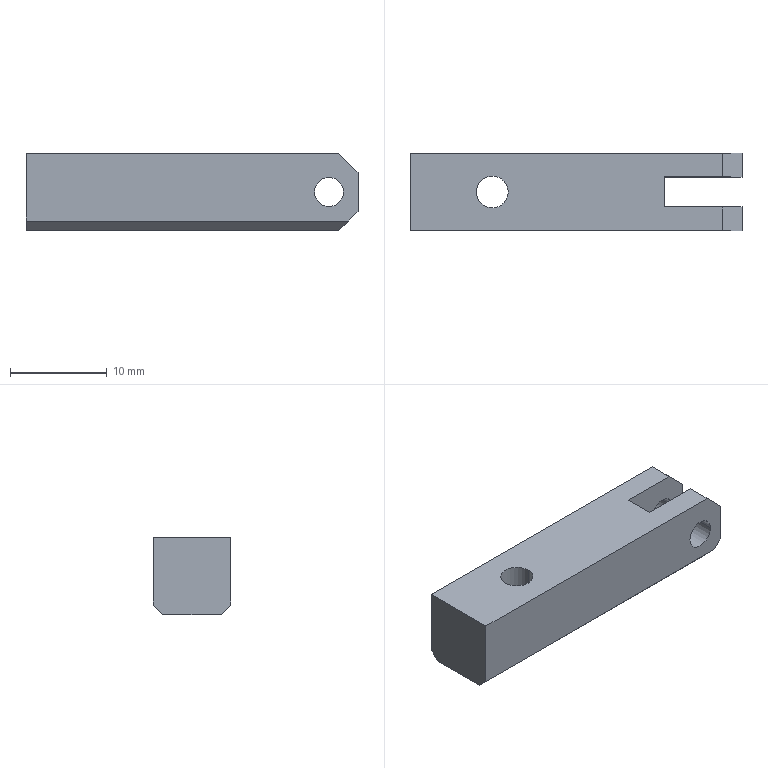Part | NX | features BREP 1 | 1 solid | 22 faces | box 34.3 x 8 x 8 mm | volume 1842 mm3 | plane 16 | cylinder 6 | commonest cylinder face diameters 3 x4 3.3 x2
STEP:
#1=CARTESIAN_POINT('',(-742.945,57.566,0.));
#2=VERTEX_POINT('',#1);
#3=CARTESIAN_POINT('',(-739.645,57.566,0.));
#4=VERTEX_POINT('',#3);
#5=CARTESIAN_POINT('',(-741.295,57.566,0.));
#6=DIRECTION('',(0.,0.,1.));
#7=DIRECTION('',(1.,0.,0.));
#8=AXIS2_PLACEMENT_3D('',#5,#6,#7);
#9=CIRCLE('',#8,1.65);
#10=EDGE_CURVE('',#2,#4,#9,.T.);
#11=ORIENTED_EDGE('',*,*,#10,.F.);
#12=CARTESIAN_POINT('',(-742.945,57.566,8.));
#13=VERTEX_POINT('',#12);
#14=CARTESIAN_POINT('',(-742.945,57.566,8.));
#15=DIRECTION('',(0.,0.,1.));
#16=VECTOR('',#15,1000.);
#17=LINE('',#14,#16);
#18=EDGE_CURVE('',#13,#2,#17,.F.);
#19=ORIENTED_EDGE('',*,*,#18,.F.);
#20=CARTESIAN_POINT('',(-739.645,57.566,8.));
#21=VERTEX_POINT('',#20);
#22=CARTESIAN_POINT('',(-741.295,57.566,8.));
#23=DIRECTION('',(0.,0.,1.));
#24=DIRECTION('',(1.,0.,0.));
#25=AXIS2_PLACEMENT_3D('',#22,#23,#24);
#26=CIRCLE('',#25,1.65);
#27=EDGE_CURVE('',#13,#21,#26,.T.);
#28=ORIENTED_EDGE('',*,*,#27,.T.);
#29=CARTESIAN_POINT('',(-739.645,57.566,8.));
#30=DIRECTION('',(0.,0.,1.));
#31=VECTOR('',#30,1000.);
#32=LINE('',#29,#31);
#33=EDGE_CURVE('',#21,#4,#32,.F.);
#34=ORIENTED_EDGE('',*,*,#33,.T.);
#35=EDGE_LOOP('',(#11,#19,#28,#34));
#36=FACE_BOUND('',#35,.T.);
#37=CARTESIAN_POINT('',(-741.295,57.566,8.));
#38=DIRECTION('',(0.,0.,1.));
#39=DIRECTION('',(1.,0.,0.));
#40=AXIS2_PLACEMENT_3D('',#37,#38,#39);
#41=CYLINDRICAL_SURFACE('',#40,1.65);
#42=ADVANCED_FACE('',(#36),#41,.F.);
#43=CARTESIAN_POINT('',(-719.995,56.016,4.));
#44=VERTEX_POINT('',#43);
#45=CARTESIAN_POINT('',(-716.995,56.016,4.));
#46=VERTEX_POINT('',#45);
#47=CARTESIAN_POINT('',(-718.495,56.016,4.));
#48=DIRECTION('',(0.,-1.,0.));
#49=DIRECTION('',(1.,0.,0.));
#50=AXIS2_PLACEMENT_3D('',#47,#48,#49);
#51=CIRCLE('',#50,1.5);
#52=EDGE_CURVE('',#44,#46,#51,.T.);
#53=ORIENTED_EDGE('',*,*,#52,.F.);
#54=CARTESIAN_POINT('',(-719.995,53.566,4.));
#55=VERTEX_POINT('',#54);
#56=CARTESIAN_POINT('',(-719.995,61.566,4.));
#57=DIRECTION('',(0.,-1.,0.));
#58=VECTOR('',#57,1000.);
#59=LINE('',#56,#58);
#60=EDGE_CURVE('',#55,#44,#59,.F.);
#61=ORIENTED_EDGE('',*,*,#60,.F.);
#62=CARTESIAN_POINT('',(-716.995,53.566,4.));
#63=VERTEX_POINT('',#62);
#64=CARTESIAN_POINT('',(-718.495,53.566,4.));
#65=DIRECTION('',(0.,-1.,0.));
#66=DIRECTION('',(1.,0.,0.));
#67=AXIS2_PLACEMENT_3D('',#64,#65,#66);
#68=CIRCLE('',#67,1.5);
#69=EDGE_CURVE('',#55,#63,#68,.T.);
#70=ORIENTED_EDGE('',*,*,#69,.T.);
#71=CARTESIAN_POINT('',(-716.995,61.566,4.));
#72=DIRECTION('',(0.,-1.,0.));
#73=VECTOR('',#72,1000.);
#74=LINE('',#71,#73);
#75=EDGE_CURVE('',#63,#46,#74,.F.);
#76=ORIENTED_EDGE('',*,*,#75,.T.);
#77=EDGE_LOOP('',(#53,#61,#70,#76));
#78=FACE_BOUND('',#77,.T.);
#79=CARTESIAN_POINT('',(-718.495,61.566,4.));
#80=DIRECTION('',(0.,-1.,0.));
#81=DIRECTION('',(1.,0.,0.));
#82=AXIS2_PLACEMENT_3D('',#79,#80,#81);
#83=CYLINDRICAL_SURFACE('',#82,1.5);
#84=ADVANCED_FACE('',(#78),#83,.F.);
#85=CARTESIAN_POINT('',(-719.995,61.566,4.));
#86=VERTEX_POINT('',#85);
#87=CARTESIAN_POINT('',(-716.995,61.566,4.));
#88=VERTEX_POINT('',#87);
#89=CARTESIAN_POINT('',(-718.495,61.566,4.));
#90=DIRECTION('',(0.,-1.,0.));
#91=DIRECTION('',(1.,0.,0.));
#92=AXIS2_PLACEMENT_3D('',#89,#90,#91);
#93=CIRCLE('',#92,1.5);
#94=EDGE_CURVE('',#86,#88,#93,.T.);
#95=ORIENTED_EDGE('',*,*,#94,.F.);
#96=CARTESIAN_POINT('',(-719.995,59.116,4.));
#97=VERTEX_POINT('',#96);
#98=CARTESIAN_POINT('',(-719.995,61.566,4.));
#99=DIRECTION('',(0.,-1.,0.));
#100=VECTOR('',#99,1000.);
#101=LINE('',#98,#100);
#102=EDGE_CURVE('',#97,#86,#101,.F.);
#103=ORIENTED_EDGE('',*,*,#102,.F.);
#104=CARTESIAN_POINT('',(-716.995,59.116,4.));
#105=VERTEX_POINT('',#104);
#106=CARTESIAN_POINT('',(-718.495,59.116,4.));
#107=DIRECTION('',(0.,1.,0.));
#108=DIRECTION('',(-1.,0.,0.));
#109=AXIS2_PLACEMENT_3D('',#106,#107,#108);
#110=CIRCLE('',#109,1.5);
#111=EDGE_CURVE('',#105,#97,#110,.T.);
#112=ORIENTED_EDGE('',*,*,#111,.F.);
#113=CARTESIAN_POINT('',(-716.995,61.566,4.));
#114=DIRECTION('',(0.,-1.,0.));
#115=VECTOR('',#114,1000.);
#116=LINE('',#113,#115);
#117=EDGE_CURVE('',#105,#88,#116,.F.);
#118=ORIENTED_EDGE('',*,*,#117,.T.);
#119=EDGE_LOOP('',(#95,#103,#112,#118));
#120=FACE_BOUND('',#119,.T.);
#121=CARTESIAN_POINT('',(-718.495,61.566,4.));
#122=DIRECTION('',(0.,-1.,0.));
#123=DIRECTION('',(1.,0.,0.));
#124=AXIS2_PLACEMENT_3D('',#121,#122,#123);
#125=CYLINDRICAL_SURFACE('',#124,1.5);
#126=ADVANCED_FACE('',(#120),#125,.F.);
#127=CARTESIAN_POINT('',(-715.495,53.566,6.));
#128=VERTEX_POINT('',#127);
#129=CARTESIAN_POINT('',(-715.495,53.566,2.));
#130=VERTEX_POINT('',#129);
#131=CARTESIAN_POINT('',(-715.495,53.566,8.));
#132=DIRECTION('',(0.,0.,-1.));
#133=VECTOR('',#132,1000.);
#134=LINE('',#131,#133);
#135=EDGE_CURVE('',#128,#130,#134,.T.);
#136=ORIENTED_EDGE('',*,*,#135,.T.);
#137=CARTESIAN_POINT('',(-715.495,56.016,2.));
#138=VERTEX_POINT('',#137);
#139=CARTESIAN_POINT('',(-715.495,53.566,2.));
#140=DIRECTION('',(0.,1.,0.));
#141=VECTOR('',#140,1000.);
#142=LINE('',#139,#141);
#143=EDGE_CURVE('',#130,#138,#142,.T.);
#144=ORIENTED_EDGE('',*,*,#143,.T.);
#145=CARTESIAN_POINT('',(-715.495,56.016,6.));
#146=VERTEX_POINT('',#145);
#147=CARTESIAN_POINT('',(-715.495,56.016,0.));
#148=DIRECTION('',(0.,0.,1.));
#149=VECTOR('',#148,1000.);
#150=LINE('',#147,#149);
#151=EDGE_CURVE('',#138,#146,#150,.T.);
#152=ORIENTED_EDGE('',*,*,#151,.T.);
#153=CARTESIAN_POINT('',(-715.495,53.566,6.));
#154=DIRECTION('',(0.,-1.,0.));
#155=VECTOR('',#154,1000.);
#156=LINE('',#153,#155);
#157=EDGE_CURVE('',#146,#128,#156,.T.);
#158=ORIENTED_EDGE('',*,*,#157,.T.);
#159=EDGE_LOOP('',(#136,#144,#152,#158));
#160=FACE_BOUND('',#159,.T.);
#161=CARTESIAN_POINT('',(-715.495,53.566,8.));
#162=DIRECTION('',(-1.,0.,0.));
#163=DIRECTION('',(0.,0.,1.));
#164=AXIS2_PLACEMENT_3D('',#161,#162,#163);
#165=PLANE('',#164);
#166=ADVANCED_FACE('',(#160),#165,.F.);
#167=CARTESIAN_POINT('',(-715.495,59.116,2.));
#168=VERTEX_POINT('',#167);
#169=CARTESIAN_POINT('',(-715.495,59.116,6.));
#170=VERTEX_POINT('',#169);
#171=CARTESIAN_POINT('',(-715.495,59.116,0.));
#172=DIRECTION('',(0.,0.,1.));
#173=VECTOR('',#172,1000.);
#174=LINE('',#171,#173);
#175=EDGE_CURVE('',#168,#170,#174,.T.);
#176=ORIENTED_EDGE('',*,*,#175,.F.);
#177=CARTESIAN_POINT('',(-715.495,61.566,2.));
#178=VERTEX_POINT('',#177);
#179=CARTESIAN_POINT('',(-715.495,53.566,2.));
#180=DIRECTION('',(0.,1.,0.));
#181=VECTOR('',#180,1000.);
#182=LINE('',#179,#181);
#183=EDGE_CURVE('',#168,#178,#182,.T.);
#184=ORIENTED_EDGE('',*,*,#183,.T.);
#185=CARTESIAN_POINT('',(-715.495,61.566,6.));
#186=VERTEX_POINT('',#185);
#187=CARTESIAN_POINT('',(-715.495,61.566,8.));
#188=DIRECTION('',(0.,0.,-1.));
#189=VECTOR('',#188,1000.);
#190=LINE('',#187,#189);
#191=EDGE_CURVE('',#186,#178,#190,.T.);
#192=ORIENTED_EDGE('',*,*,#191,.F.);
#193=CARTESIAN_POINT('',(-715.495,59.116,6.));
#194=DIRECTION('',(0.,-1.,0.));
#195=VECTOR('',#194,1000.);
#196=LINE('',#193,#195);
#197=EDGE_CURVE('',#186,#170,#196,.T.);
#198=ORIENTED_EDGE('',*,*,#197,.T.);
#199=EDGE_LOOP('',(#176,#184,#192,#198));
#200=FACE_BOUND('',#199,.T.);
#201=CARTESIAN_POINT('',(-715.495,53.566,8.));
#202=DIRECTION('',(-1.,0.,0.));
#203=DIRECTION('',(0.,0.,1.));
#204=AXIS2_PLACEMENT_3D('',#201,#202,#203);
#205=PLANE('',#204);
#206=ADVANCED_FACE('',(#200),#205,.F.);
#207=CARTESIAN_POINT('',(-716.495,61.566,1.));
#208=VERTEX_POINT('',#207);
#209=CARTESIAN_POINT('',(-715.495,61.566,2.));
#210=DIRECTION('',(-0.7071,0.,-0.7071));
#211=VECTOR('',#210,1000.);
#212=LINE('',#209,#211);
#213=EDGE_CURVE('',#178,#208,#212,.T.);
#214=ORIENTED_EDGE('',*,*,#213,.T.);
#215=CARTESIAN_POINT('',(-749.795,61.566,1.));
#216=VERTEX_POINT('',#215);
#217=CARTESIAN_POINT('',(-715.495,61.566,1.));
#218=DIRECTION('',(-1.,0.,0.));
#219=VECTOR('',#218,1000.);
#220=LINE('',#217,#219);
#221=EDGE_CURVE('',#208,#216,#220,.T.);
#222=ORIENTED_EDGE('',*,*,#221,.T.);
#223=CARTESIAN_POINT('',(-749.795,61.566,8.));
#224=VERTEX_POINT('',#223);
#225=CARTESIAN_POINT('',(-749.795,61.566,8.));
#226=DIRECTION('',(0.,0.,-1.));
#227=VECTOR('',#226,1000.);
#228=LINE('',#225,#227);
#229=EDGE_CURVE('',#224,#216,#228,.T.);
#230=ORIENTED_EDGE('',*,*,#229,.F.);
#231=CARTESIAN_POINT('',(-717.495,61.566,8.));
#232=VERTEX_POINT('',#231);
#233=CARTESIAN_POINT('',(-715.495,61.566,8.));
#234=DIRECTION('',(-1.,0.,0.));
#235=VECTOR('',#234,1000.);
#236=LINE('',#233,#235);
#237=EDGE_CURVE('',#232,#224,#236,.T.);
#238=ORIENTED_EDGE('',*,*,#237,.F.);
#239=CARTESIAN_POINT('',(-717.495,61.566,8.));
#240=DIRECTION('',(0.7071,0.,-0.7071));
#241=VECTOR('',#240,1000.);
#242=LINE('',#239,#241);
#243=EDGE_CURVE('',#232,#186,#242,.T.);
#244=ORIENTED_EDGE('',*,*,#243,.T.);
#245=ORIENTED_EDGE('',*,*,#191,.T.);
#246=EDGE_LOOP('',(#214,#222,#230,#238,#244,#245));
#247=FACE_BOUND('',#246,.T.);
#248=CARTESIAN_POINT('',(-718.495,61.566,4.));
#249=DIRECTION('',(0.,-1.,0.));
#250=DIRECTION('',(1.,0.,0.));
#251=AXIS2_PLACEMENT_3D('',#248,#249,#250);
#252=CIRCLE('',#251,1.5);
#253=EDGE_CURVE('',#88,#86,#252,.T.);
#254=ORIENTED_EDGE('',*,*,#253,.T.);
#255=ORIENTED_EDGE('',*,*,#94,.T.);
#256=EDGE_LOOP('',(#254,#255));
#257=FACE_BOUND('',#256,.T.);
#258=CARTESIAN_POINT('',(-715.495,61.566,8.));
#259=DIRECTION('',(0.,-1.,0.));
#260=DIRECTION('',(0.,0.,-1.));
#261=AXIS2_PLACEMENT_3D('',#258,#259,#260);
#262=PLANE('',#261);
#263=ADVANCED_FACE('',(#247,#257),#262,.F.);
#264=CARTESIAN_POINT('',(-749.795,60.566,0.));
#265=VERTEX_POINT('',#264);
#266=CARTESIAN_POINT('',(-749.795,54.566,0.));
#267=VERTEX_POINT('',#266);
#268=CARTESIAN_POINT('',(-749.795,53.566,0.));
#269=DIRECTION('',(0.,-1.,0.));
#270=VECTOR('',#269,1000.);
#271=LINE('',#268,#270);
#272=EDGE_CURVE('',#265,#267,#271,.T.);
#273=ORIENTED_EDGE('',*,*,#272,.T.);
#274=CARTESIAN_POINT('',(-749.795,53.566,1.));
#275=VERTEX_POINT('',#274);
#276=CARTESIAN_POINT('',(-749.795,53.566,1.));
#277=DIRECTION('',(0.,-0.7071,0.7071));
#278=VECTOR('',#277,1000.);
#279=LINE('',#276,#278);
#280=EDGE_CURVE('',#267,#275,#279,.T.);
#281=ORIENTED_EDGE('',*,*,#280,.T.);
#282=CARTESIAN_POINT('',(-749.795,53.566,8.));
#283=VERTEX_POINT('',#282);
#284=CARTESIAN_POINT('',(-749.795,53.566,8.));
#285=DIRECTION('',(0.,0.,-1.));
#286=VECTOR('',#285,1000.);
#287=LINE('',#284,#286);
#288=EDGE_CURVE('',#283,#275,#287,.T.);
#289=ORIENTED_EDGE('',*,*,#288,.F.);
#290=CARTESIAN_POINT('',(-749.795,53.566,8.));
#291=DIRECTION('',(0.,-1.,0.));
#292=VECTOR('',#291,1000.);
#293=LINE('',#290,#292);
#294=EDGE_CURVE('',#224,#283,#293,.T.);
#295=ORIENTED_EDGE('',*,*,#294,.F.);
#296=ORIENTED_EDGE('',*,*,#229,.T.);
#297=CARTESIAN_POINT('',(-749.795,61.566,1.));
#298=DIRECTION('',(0.,-0.7071,-0.7071));
#299=VECTOR('',#298,1000.);
#300=LINE('',#297,#299);
#301=EDGE_CURVE('',#216,#265,#300,.T.);
#302=ORIENTED_EDGE('',*,*,#301,.T.);
#303=EDGE_LOOP('',(#273,#281,#289,#295,#296,#302));
#304=FACE_BOUND('',#303,.T.);
#305=CARTESIAN_POINT('',(-749.795,53.566,8.));
#306=DIRECTION('',(1.,0.,0.));
#307=DIRECTION('',(0.,1.,0.));
#308=AXIS2_PLACEMENT_3D('',#305,#306,#307);
#309=PLANE('',#308);
#310=ADVANCED_FACE('',(#304),#309,.F.);
#311=ORIENTED_EDGE('',*,*,#288,.T.);
#312=CARTESIAN_POINT('',(-716.495,53.566,1.));
#313=VERTEX_POINT('',#312);
#314=CARTESIAN_POINT('',(-715.495,53.566,1.));
#315=DIRECTION('',(1.,0.,0.));
#316=VECTOR('',#315,1000.);
#317=LINE('',#314,#316);
#318=EDGE_CURVE('',#275,#313,#317,.T.);
#319=ORIENTED_EDGE('',*,*,#318,.T.);
#320=CARTESIAN_POINT('',(-715.495,53.566,2.));
#321=DIRECTION('',(0.7071,0.,0.7071));
#322=VECTOR('',#321,1000.);
#323=LINE('',#320,#322);
#324=EDGE_CURVE('',#313,#130,#323,.T.);
#325=ORIENTED_EDGE('',*,*,#324,.T.);
#326=ORIENTED_EDGE('',*,*,#135,.F.);
#327=CARTESIAN_POINT('',(-717.495,53.566,8.));
#328=VERTEX_POINT('',#327);
#329=CARTESIAN_POINT('',(-717.495,53.566,8.));
#330=DIRECTION('',(-0.7071,0.,0.7071));
#331=VECTOR('',#330,1000.);
#332=LINE('',#329,#331);
#333=EDGE_CURVE('',#128,#328,#332,.T.);
#334=ORIENTED_EDGE('',*,*,#333,.T.);
#335=CARTESIAN_POINT('',(-715.495,53.566,8.));
#336=DIRECTION('',(1.,0.,0.));
#337=VECTOR('',#336,1000.);
#338=LINE('',#335,#337);
#339=EDGE_CURVE('',#283,#328,#338,.T.);
#340=ORIENTED_EDGE('',*,*,#339,.F.);
#341=EDGE_LOOP('',(#311,#319,#325,#326,#334,#340));
#342=FACE_BOUND('',#341,.T.);
#343=CARTESIAN_POINT('',(-718.495,53.566,4.));
#344=DIRECTION('',(0.,-1.,0.));
#345=DIRECTION('',(1.,0.,0.));
#346=AXIS2_PLACEMENT_3D('',#343,#344,#345);
#347=CIRCLE('',#346,1.5);
#348=EDGE_CURVE('',#63,#55,#347,.T.);
#349=ORIENTED_EDGE('',*,*,#348,.F.);
#350=ORIENTED_EDGE('',*,*,#69,.F.);
#351=EDGE_LOOP('',(#349,#350));
#352=FACE_BOUND('',#351,.T.);
#353=CARTESIAN_POINT('',(-715.495,53.566,8.));
#354=DIRECTION('',(0.,1.,0.));
#355=DIRECTION('',(1.,0.,0.));
#356=AXIS2_PLACEMENT_3D('',#353,#354,#355);
#357=PLANE('',#356);
#358=ADVANCED_FACE('',(#342,#352),#357,.F.);
#359=ORIENTED_EDGE('',*,*,#339,.T.);
#360=CARTESIAN_POINT('',(-717.495,56.016,8.));
#361=VERTEX_POINT('',#360);
#362=CARTESIAN_POINT('',(-717.495,56.016,8.));
#363=DIRECTION('',(0.,1.,0.));
#364=VECTOR('',#363,1000.);
#365=LINE('',#362,#364);
#366=EDGE_CURVE('',#328,#361,#365,.T.);
#367=ORIENTED_EDGE('',*,*,#366,.T.);
#368=CARTESIAN_POINT('',(-723.495,56.016,8.));
#369=VERTEX_POINT('',#368);
#370=CARTESIAN_POINT('',(-715.495,56.016,8.));
#371=DIRECTION('',(1.,0.,0.));
#372=VECTOR('',#371,1000.);
#373=LINE('',#370,#372);
#374=EDGE_CURVE('',#369,#361,#373,.T.);
#375=ORIENTED_EDGE('',*,*,#374,.F.);
#376=CARTESIAN_POINT('',(-723.495,59.116,8.));
#377=VERTEX_POINT('',#376);
#378=CARTESIAN_POINT('',(-723.495,56.016,8.));
#379=DIRECTION('',(0.,-1.,0.));
#380=VECTOR('',#379,1000.);
#381=LINE('',#378,#380);
#382=EDGE_CURVE('',#377,#369,#381,.T.);
#383=ORIENTED_EDGE('',*,*,#382,.F.);
#384=CARTESIAN_POINT('',(-717.495,59.116,8.));
#385=VERTEX_POINT('',#384);
#386=CARTESIAN_POINT('',(-715.495,59.116,8.));
#387=DIRECTION('',(-1.,0.,0.));
#388=VECTOR('',#387,1000.);
#389=LINE('',#386,#388);
#390=EDGE_CURVE('',#385,#377,#389,.T.);
#391=ORIENTED_EDGE('',*,*,#390,.F.);
#392=CARTESIAN_POINT('',(-717.495,61.566,8.));
#393=DIRECTION('',(0.,1.,0.));
#394=VECTOR('',#393,1000.);
#395=LINE('',#392,#394);
#396=EDGE_CURVE('',#385,#232,#395,.T.);
#397=ORIENTED_EDGE('',*,*,#396,.T.);
#398=ORIENTED_EDGE('',*,*,#237,.T.);
#399=ORIENTED_EDGE('',*,*,#294,.T.);
#400=EDGE_LOOP('',(#359,#367,#375,#383,#391,#397,#398,#399));
#401=FACE_BOUND('',#400,.T.);
#402=CARTESIAN_POINT('',(-741.295,57.566,8.));
#403=DIRECTION('',(0.,0.,1.));
#404=DIRECTION('',(1.,0.,0.));
#405=AXIS2_PLACEMENT_3D('',#402,#403,#404);
#406=CIRCLE('',#405,1.65);
#407=EDGE_CURVE('',#21,#13,#406,.T.);
#408=ORIENTED_EDGE('',*,*,#407,.F.);
#409=ORIENTED_EDGE('',*,*,#27,.F.);
#410=EDGE_LOOP('',(#408,#409));
#411=FACE_BOUND('',#410,.T.);
#412=CARTESIAN_POINT('',(-715.495,61.566,8.));
#413=DIRECTION('',(0.,0.,1.));
#414=DIRECTION('',(1.,0.,0.));
#415=AXIS2_PLACEMENT_3D('',#412,#413,#414);
#416=PLANE('',#415);
#417=ADVANCED_FACE('',(#401,#411),#416,.T.);
#418=CARTESIAN_POINT('',(-717.495,56.016,0.));
#419=VERTEX_POINT('',#418);
#420=CARTESIAN_POINT('',(-717.495,54.566,0.));
#421=VERTEX_POINT('',#420);
#422=CARTESIAN_POINT('',(-717.495,61.566,0.));
#423=DIRECTION('',(0.,-1.,0.));
#424=VECTOR('',#423,1000.);
#425=LINE('',#422,#424);
#426=EDGE_CURVE('',#419,#421,#425,.T.);
#427=ORIENTED_EDGE('',*,*,#426,.T.);
#428=CARTESIAN_POINT('',(-715.495,54.566,0.));
#429=DIRECTION('',(-1.,0.,0.));
#430=VECTOR('',#429,1000.);
#431=LINE('',#428,#430);
#432=EDGE_CURVE('',#421,#267,#431,.T.);
#433=ORIENTED_EDGE('',*,*,#432,.T.);
#434=ORIENTED_EDGE('',*,*,#272,.F.);
#435=CARTESIAN_POINT('',(-717.495,60.566,0.));
#436=VERTEX_POINT('',#435);
#437=CARTESIAN_POINT('',(-715.495,60.566,0.));
#438=DIRECTION('',(1.,0.,0.));
#439=VECTOR('',#438,1000.);
#440=LINE('',#437,#439);
#441=EDGE_CURVE('',#265,#436,#440,.T.);
#442=ORIENTED_EDGE('',*,*,#441,.T.);
#443=CARTESIAN_POINT('',(-717.495,59.116,0.));
#444=VERTEX_POINT('',#443);
#445=CARTESIAN_POINT('',(-717.495,61.566,0.));
#446=DIRECTION('',(0.,-1.,0.));
#447=VECTOR('',#446,1000.);
#448=LINE('',#445,#447);
#449=EDGE_CURVE('',#436,#444,#448,.T.);
#450=ORIENTED_EDGE('',*,*,#449,.T.);
#451=CARTESIAN_POINT('',(-723.495,59.116,0.));
#452=VERTEX_POINT('',#451);
#453=CARTESIAN_POINT('',(-715.495,59.116,0.));
#454=DIRECTION('',(-1.,0.,0.));
#455=VECTOR('',#454,1000.);
#456=LINE('',#453,#455);
#457=EDGE_CURVE('',#444,#452,#456,.T.);
#458=ORIENTED_EDGE('',*,*,#457,.T.);
#459=CARTESIAN_POINT('',(-723.495,56.016,0.));
#460=VERTEX_POINT('',#459);
#461=CARTESIAN_POINT('',(-723.495,56.016,0.));
#462=DIRECTION('',(0.,-1.,0.));
#463=VECTOR('',#462,1000.);
#464=LINE('',#461,#463);
#465=EDGE_CURVE('',#452,#460,#464,.T.);
#466=ORIENTED_EDGE('',*,*,#465,.T.);
#467=CARTESIAN_POINT('',(-715.495,56.016,0.));
#468=DIRECTION('',(1.,0.,0.));
#469=VECTOR('',#468,1000.);
#470=LINE('',#467,#469);
#471=EDGE_CURVE('',#460,#419,#470,.T.);
#472=ORIENTED_EDGE('',*,*,#471,.T.);
#473=EDGE_LOOP('',(#427,#433,#434,#442,#450,#458,#466,#472));
#474=FACE_BOUND('',#473,.T.);
#475=CARTESIAN_POINT('',(-741.295,57.566,0.));
#476=DIRECTION('',(0.,0.,1.));
#477=DIRECTION('',(1.,0.,0.));
#478=AXIS2_PLACEMENT_3D('',#475,#476,#477);
#479=CIRCLE('',#478,1.65);
#480=EDGE_CURVE('',#4,#2,#479,.T.);
#481=ORIENTED_EDGE('',*,*,#480,.T.);
#482=ORIENTED_EDGE('',*,*,#10,.T.);
#483=EDGE_LOOP('',(#481,#482));
#484=FACE_BOUND('',#483,.T.);
#485=CARTESIAN_POINT('',(-715.495,61.566,0.));
#486=DIRECTION('',(0.,0.,1.));
#487=DIRECTION('',(1.,0.,0.));
#488=AXIS2_PLACEMENT_3D('',#485,#486,#487);
#489=PLANE('',#488);
#490=ADVANCED_FACE('',(#474,#484),#489,.F.);
#491=ORIENTED_EDGE('',*,*,#151,.F.);
#492=CARTESIAN_POINT('',(-715.495,56.016,2.));
#493=DIRECTION('',(-0.7071,0.,-0.7071));
#494=VECTOR('',#493,1000.);
#495=LINE('',#492,#494);
#496=EDGE_CURVE('',#138,#419,#495,.T.);
#497=ORIENTED_EDGE('',*,*,#496,.T.);
#498=ORIENTED_EDGE('',*,*,#471,.F.);
#499=CARTESIAN_POINT('',(-723.495,56.016,0.));
#500=DIRECTION('',(0.,0.,1.));
#501=VECTOR('',#500,1000.);
#502=LINE('',#499,#501);
#503=EDGE_CURVE('',#460,#369,#502,.T.);
#504=ORIENTED_EDGE('',*,*,#503,.T.);
#505=ORIENTED_EDGE('',*,*,#374,.T.);
#506=CARTESIAN_POINT('',(-717.495,56.016,8.));
#507=DIRECTION('',(0.7071,0.,-0.7071));
#508=VECTOR('',#507,1000.);
#509=LINE('',#506,#508);
#510=EDGE_CURVE('',#361,#146,#509,.T.);
#511=ORIENTED_EDGE('',*,*,#510,.T.);
#512=EDGE_LOOP('',(#491,#497,#498,#504,#505,#511));
#513=FACE_BOUND('',#512,.T.);
#514=CARTESIAN_POINT('',(-718.495,56.016,4.));
#515=DIRECTION('',(0.,-1.,0.));
#516=DIRECTION('',(1.,0.,0.));
#517=AXIS2_PLACEMENT_3D('',#514,#515,#516);
#518=CIRCLE('',#517,1.5);
#519=EDGE_CURVE('',#46,#44,#518,.T.);
#520=ORIENTED_EDGE('',*,*,#519,.T.);
#521=ORIENTED_EDGE('',*,*,#52,.T.);
#522=EDGE_LOOP('',(#520,#521));
#523=FACE_BOUND('',#522,.T.);
#524=CARTESIAN_POINT('',(-715.495,56.016,0.));
#525=DIRECTION('',(0.,-1.,0.));
#526=DIRECTION('',(0.,0.,-1.));
#527=AXIS2_PLACEMENT_3D('',#524,#525,#526);
#528=PLANE('',#527);
#529=ADVANCED_FACE('',(#513,#523),#528,.F.);
#530=ORIENTED_EDGE('',*,*,#382,.T.);
#531=ORIENTED_EDGE('',*,*,#503,.F.);
#532=ORIENTED_EDGE('',*,*,#465,.F.);
#533=CARTESIAN_POINT('',(-723.495,59.116,0.));
#534=DIRECTION('',(0.,0.,1.));
#535=VECTOR('',#534,1000.);
#536=LINE('',#533,#535);
#537=EDGE_CURVE('',#452,#377,#536,.T.);
#538=ORIENTED_EDGE('',*,*,#537,.T.);
#539=EDGE_LOOP('',(#530,#531,#532,#538));
#540=FACE_BOUND('',#539,.T.);
#541=CARTESIAN_POINT('',(-723.495,56.016,0.));
#542=DIRECTION('',(-1.,0.,0.));
#543=DIRECTION('',(0.,0.,1.));
#544=AXIS2_PLACEMENT_3D('',#541,#542,#543);
#545=PLANE('',#544);
#546=ADVANCED_FACE('',(#540),#545,.F.);
#547=ORIENTED_EDGE('',*,*,#457,.F.);
#548=CARTESIAN_POINT('',(-715.495,59.116,2.));
#549=DIRECTION('',(0.7071,0.,0.7071));
#550=VECTOR('',#549,1000.);
#551=LINE('',#548,#550);
#552=EDGE_CURVE('',#444,#168,#551,.T.);
#553=ORIENTED_EDGE('',*,*,#552,.T.);
#554=ORIENTED_EDGE('',*,*,#175,.T.);
#555=CARTESIAN_POINT('',(-717.495,59.116,8.));
#556=DIRECTION('',(-0.7071,0.,0.7071));
#557=VECTOR('',#556,1000.);
#558=LINE('',#555,#557);
#559=EDGE_CURVE('',#170,#385,#558,.T.);
#560=ORIENTED_EDGE('',*,*,#559,.T.);
#561=ORIENTED_EDGE('',*,*,#390,.T.);
#562=ORIENTED_EDGE('',*,*,#537,.F.);
#563=EDGE_LOOP('',(#547,#553,#554,#560,#561,#562));
#564=FACE_BOUND('',#563,.T.);
#565=ORIENTED_EDGE('',*,*,#111,.T.);
#566=CARTESIAN_POINT('',(-718.495,59.116,4.));
#567=DIRECTION('',(0.,1.,0.));
#568=DIRECTION('',(-1.,0.,0.));
#569=AXIS2_PLACEMENT_3D('',#566,#567,#568);
#570=CIRCLE('',#569,1.5);
#571=EDGE_CURVE('',#97,#105,#570,.T.);
#572=ORIENTED_EDGE('',*,*,#571,.T.);
#573=EDGE_LOOP('',(#565,#572));
#574=FACE_BOUND('',#573,.T.);
#575=CARTESIAN_POINT('',(-715.495,59.116,0.));
#576=DIRECTION('',(0.,1.,0.));
#577=DIRECTION('',(1.,0.,0.));
#578=AXIS2_PLACEMENT_3D('',#575,#576,#577);
#579=PLANE('',#578);
#580=ADVANCED_FACE('',(#564,#574),#579,.F.);
#581=ORIENTED_EDGE('',*,*,#102,.T.);
#582=ORIENTED_EDGE('',*,*,#253,.F.);
#583=ORIENTED_EDGE('',*,*,#117,.F.);
#584=ORIENTED_EDGE('',*,*,#571,.F.);
#585=EDGE_LOOP('',(#581,#582,#583,#584));
#586=FACE_BOUND('',#585,.T.);
#587=CARTESIAN_POINT('',(-718.495,61.566,4.));
#588=DIRECTION('',(0.,-1.,0.));
#589=DIRECTION('',(1.,0.,0.));
#590=AXIS2_PLACEMENT_3D('',#587,#588,#589);
#591=CYLINDRICAL_SURFACE('',#590,1.5);
#592=ADVANCED_FACE('',(#586),#591,.F.);
#593=ORIENTED_EDGE('',*,*,#60,.T.);
#594=ORIENTED_EDGE('',*,*,#519,.F.);
#595=ORIENTED_EDGE('',*,*,#75,.F.);
#596=ORIENTED_EDGE('',*,*,#348,.T.);
#597=EDGE_LOOP('',(#593,#594,#595,#596));
#598=FACE_BOUND('',#597,.T.);
#599=CARTESIAN_POINT('',(-718.495,61.566,4.));
#600=DIRECTION('',(0.,-1.,0.));
#601=DIRECTION('',(1.,0.,0.));
#602=AXIS2_PLACEMENT_3D('',#599,#600,#601);
#603=CYLINDRICAL_SURFACE('',#602,1.5);
#604=ADVANCED_FACE('',(#598),#603,.F.);
#605=ORIENTED_EDGE('',*,*,#324,.F.);
#606=CARTESIAN_POINT('',(-715.828,52.899,1.667));
#607=DIRECTION('',(-0.5774,0.5774,-0.5774));
#608=VECTOR('',#607,1000.);
#609=LINE('',#606,#608);
#610=EDGE_CURVE('',#313,#421,#609,.T.);
#611=ORIENTED_EDGE('',*,*,#610,.T.);
#612=ORIENTED_EDGE('',*,*,#426,.F.);
#613=ORIENTED_EDGE('',*,*,#496,.F.);
#614=ORIENTED_EDGE('',*,*,#143,.F.);
#615=EDGE_LOOP('',(#605,#611,#612,#613,#614));
#616=FACE_BOUND('',#615,.T.);
#617=CARTESIAN_POINT('',(-715.495,53.566,2.));
#618=DIRECTION('',(-0.7071,0.,0.7071));
#619=DIRECTION('',(0.,1.,0.));
#620=AXIS2_PLACEMENT_3D('',#617,#618,#619);
#621=PLANE('',#620);
#622=ADVANCED_FACE('',(#616),#621,.F.);
#623=ORIENTED_EDGE('',*,*,#449,.F.);
#624=CARTESIAN_POINT('',(-718.495,59.566,-1.));
#625=DIRECTION('',(0.5774,0.5774,0.5774));
#626=VECTOR('',#625,1000.);
#627=LINE('',#624,#626);
#628=EDGE_CURVE('',#436,#208,#627,.T.);
#629=ORIENTED_EDGE('',*,*,#628,.T.);
#630=ORIENTED_EDGE('',*,*,#213,.F.);
#631=ORIENTED_EDGE('',*,*,#183,.F.);
#632=ORIENTED_EDGE('',*,*,#552,.F.);
#633=EDGE_LOOP('',(#623,#629,#630,#631,#632));
#634=FACE_BOUND('',#633,.T.);
#635=CARTESIAN_POINT('',(-715.495,53.566,2.));
#636=DIRECTION('',(-0.7071,0.,0.7071));
#637=DIRECTION('',(0.,1.,0.));
#638=AXIS2_PLACEMENT_3D('',#635,#636,#637);
#639=PLANE('',#638);
#640=ADVANCED_FACE('',(#634),#639,.F.);
#641=ORIENTED_EDGE('',*,*,#333,.F.);
#642=ORIENTED_EDGE('',*,*,#157,.F.);
#643=ORIENTED_EDGE('',*,*,#510,.F.);
#644=ORIENTED_EDGE('',*,*,#366,.F.);
#645=EDGE_LOOP('',(#641,#642,#643,#644));
#646=FACE_BOUND('',#645,.T.);
#647=CARTESIAN_POINT('',(-717.495,61.566,8.));
#648=DIRECTION('',(0.7071,0.,0.7071));
#649=DIRECTION('',(0.,-1.,0.));
#650=AXIS2_PLACEMENT_3D('',#647,#648,#649);
#651=PLANE('',#650);
#652=ADVANCED_FACE('',(#646),#651,.T.);
#653=ORIENTED_EDGE('',*,*,#559,.F.);
#654=ORIENTED_EDGE('',*,*,#197,.F.);
#655=ORIENTED_EDGE('',*,*,#243,.F.);
#656=ORIENTED_EDGE('',*,*,#396,.F.);
#657=EDGE_LOOP('',(#653,#654,#655,#656));
#658=FACE_BOUND('',#657,.T.);
#659=CARTESIAN_POINT('',(-717.495,61.566,8.));
#660=DIRECTION('',(0.7071,0.,0.7071));
#661=DIRECTION('',(0.,-1.,0.));
#662=AXIS2_PLACEMENT_3D('',#659,#660,#661);
#663=PLANE('',#662);
#664=ADVANCED_FACE('',(#658),#663,.T.);
#665=ORIENTED_EDGE('',*,*,#280,.F.);
#666=ORIENTED_EDGE('',*,*,#432,.F.);
#667=ORIENTED_EDGE('',*,*,#610,.F.);
#668=ORIENTED_EDGE('',*,*,#318,.F.);
#669=EDGE_LOOP('',(#665,#666,#667,#668));
#670=FACE_BOUND('',#669,.T.);
#671=CARTESIAN_POINT('',(-715.495,53.566,1.));
#672=DIRECTION('',(0.,0.7071,0.7071));
#673=DIRECTION('',(1.,0.,0.));
#674=AXIS2_PLACEMENT_3D('',#671,#672,#673);
#675=PLANE('',#674);
#676=ADVANCED_FACE('',(#670),#675,.F.);
#677=ORIENTED_EDGE('',*,*,#628,.F.);
#678=ORIENTED_EDGE('',*,*,#441,.F.);
#679=ORIENTED_EDGE('',*,*,#301,.F.);
#680=ORIENTED_EDGE('',*,*,#221,.F.);
#681=EDGE_LOOP('',(#677,#678,#679,#680));
#682=FACE_BOUND('',#681,.T.);
#683=CARTESIAN_POINT('',(-715.495,61.566,1.));
#684=DIRECTION('',(0.,-0.7071,0.7071));
#685=DIRECTION('',(-1.,0.,0.));
#686=AXIS2_PLACEMENT_3D('',#683,#684,#685);
#687=PLANE('',#686);
#688=ADVANCED_FACE('',(#682),#687,.F.);
#689=ORIENTED_EDGE('',*,*,#18,.T.);
#690=ORIENTED_EDGE('',*,*,#480,.F.);
#691=ORIENTED_EDGE('',*,*,#33,.F.);
#692=ORIENTED_EDGE('',*,*,#407,.T.);
#693=EDGE_LOOP('',(#689,#690,#691,#692));
#694=FACE_BOUND('',#693,.T.);
#695=CARTESIAN_POINT('',(-741.295,57.566,8.));
#696=DIRECTION('',(0.,0.,1.));
#697=DIRECTION('',(1.,0.,0.));
#698=AXIS2_PLACEMENT_3D('',#695,#696,#697);
#699=CYLINDRICAL_SURFACE('',#698,1.65);
#700=ADVANCED_FACE('',(#694),#699,.F.);
#701=CLOSED_SHELL('',(#42,#84,#126,#166,#206,#263,#310,#358,#417,#490,#529,#546,#580,#592,#604,#622,#640,#652,#664,#676,#688,#700));
#702=MANIFOLD_SOLID_BREP('',#701);
#703=(LENGTH_UNIT()NAMED_UNIT(*)SI_UNIT(.MILLI.,.METRE.));
#704=UNCERTAINTY_MEASURE_WITH_UNIT(LENGTH_MEASURE(0.00001),#703,'','');
#705=(NAMED_UNIT(*)PLANE_ANGLE_UNIT()SI_UNIT($,.RADIAN.));
#706=(NAMED_UNIT(*)SI_UNIT($,.STERADIAN.)SOLID_ANGLE_UNIT());
#707=(GEOMETRIC_REPRESENTATION_CONTEXT(3)GLOBAL_UNCERTAINTY_ASSIGNED_CONTEXT((#704))GLOBAL_UNIT_ASSIGNED_CONTEXT((#703,#705,#706))REPRESENTATION_CONTEXT('',''));
#708=ADVANCED_BREP_SHAPE_REPRESENTATION('',(#702),#707);